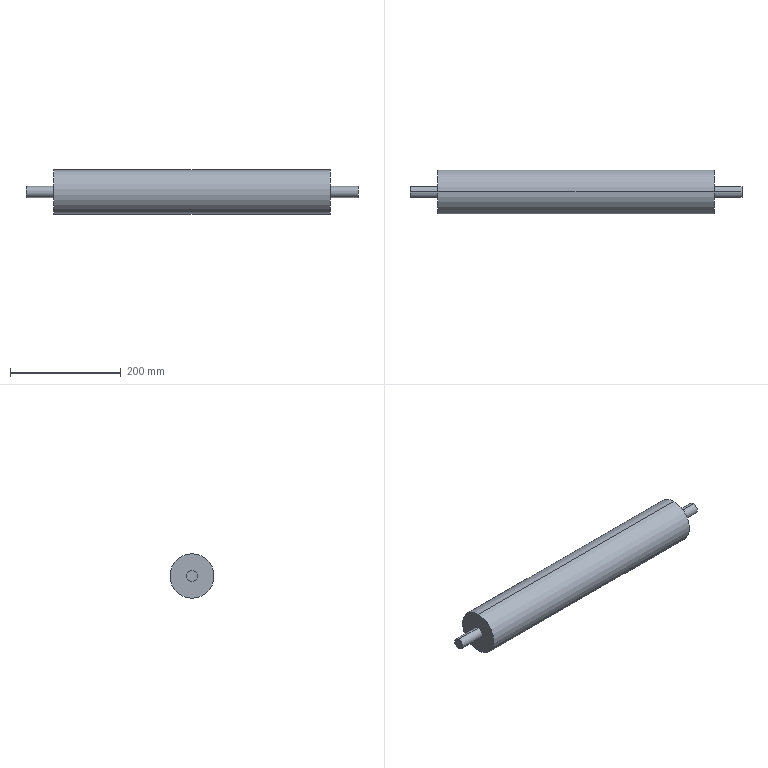Part | SolidWorks | features Revolution 1 | 1 solid | 10 faces | box 600 x 80 x 80 mm | volume 2544690 mm3 | cylinder 6 | plane 4 | commonest cylinder face diameters 20 x4 80 x2
STEP:
#1=CARTESIAN_POINT('',(-173.025,190.414,10.));
#2=VERTEX_POINT('',#1);
#3=CARTESIAN_POINT('',(-173.025,190.414,-10.));
#4=VERTEX_POINT('',#3);
#5=CARTESIAN_POINT('',(-173.025,190.414,0.));
#6=DIRECTION('',(-1.,0.,0.));
#7=DIRECTION('',(0.,0.,1.));
#8=AXIS2_PLACEMENT_3D('',#5,#6,#7);
#9=CIRCLE('',#8,10.);
#10=EDGE_CURVE('',#2,#4,#9,.T.);
#11=ORIENTED_EDGE('',*,*,#10,.T.);
#12=CARTESIAN_POINT('',(-223.025,190.414,-10.));
#13=VERTEX_POINT('',#12);
#14=CARTESIAN_POINT('',(-223.025,190.414,-10.));
#15=DIRECTION('',(-1.,0.,0.));
#16=VECTOR('',#15,1000.);
#17=LINE('',#14,#16);
#18=EDGE_CURVE('',#4,#13,#17,.T.);
#19=ORIENTED_EDGE('',*,*,#18,.T.);
#20=CARTESIAN_POINT('',(-223.025,190.414,10.));
#21=VERTEX_POINT('',#20);
#22=CARTESIAN_POINT('',(-223.025,190.414,0.));
#23=DIRECTION('',(-1.,0.,0.));
#24=DIRECTION('',(0.,0.,1.));
#25=AXIS2_PLACEMENT_3D('',#22,#23,#24);
#26=CIRCLE('',#25,10.);
#27=EDGE_CURVE('',#21,#13,#26,.T.);
#28=ORIENTED_EDGE('',*,*,#27,.F.);
#29=CARTESIAN_POINT('',(-223.025,190.414,10.));
#30=DIRECTION('',(-1.,0.,0.));
#31=VECTOR('',#30,1000.);
#32=LINE('',#29,#31);
#33=EDGE_CURVE('',#2,#21,#32,.T.);
#34=ORIENTED_EDGE('',*,*,#33,.F.);
#35=EDGE_LOOP('',(#11,#19,#28,#34));
#36=FACE_OUTER_BOUND('',#35,.T.);
#37=CARTESIAN_POINT('',(-223.025,190.414,0.));
#38=DIRECTION('',(-1.,0.,0.));
#39=DIRECTION('',(0.,0.,1.));
#40=AXIS2_PLACEMENT_3D('',#37,#38,#39);
#41=CYLINDRICAL_SURFACE('',#40,10.);
#42=ADVANCED_FACE('',(#36),#41,.T.);
#43=CARTESIAN_POINT('',(326.975,190.414,40.));
#44=VERTEX_POINT('',#43);
#45=CARTESIAN_POINT('',(326.975,190.414,-40.));
#46=VERTEX_POINT('',#45);
#47=CARTESIAN_POINT('',(326.975,190.414,0.));
#48=DIRECTION('',(-1.,0.,0.));
#49=DIRECTION('',(0.,0.,1.));
#50=AXIS2_PLACEMENT_3D('',#47,#48,#49);
#51=CIRCLE('',#50,40.);
#52=EDGE_CURVE('',#44,#46,#51,.T.);
#53=ORIENTED_EDGE('',*,*,#52,.T.);
#54=CARTESIAN_POINT('',(-173.025,190.414,-40.));
#55=VERTEX_POINT('',#54);
#56=CARTESIAN_POINT('',(-223.025,190.414,-40.));
#57=DIRECTION('',(-1.,0.,0.));
#58=VECTOR('',#57,1000.);
#59=LINE('',#56,#58);
#60=EDGE_CURVE('',#46,#55,#59,.T.);
#61=ORIENTED_EDGE('',*,*,#60,.T.);
#62=CARTESIAN_POINT('',(-173.025,190.414,40.));
#63=VERTEX_POINT('',#62);
#64=CARTESIAN_POINT('',(-173.025,190.414,0.));
#65=DIRECTION('',(-1.,0.,0.));
#66=DIRECTION('',(0.,0.,1.));
#67=AXIS2_PLACEMENT_3D('',#64,#65,#66);
#68=CIRCLE('',#67,40.);
#69=EDGE_CURVE('',#63,#55,#68,.T.);
#70=ORIENTED_EDGE('',*,*,#69,.F.);
#71=CARTESIAN_POINT('',(-223.025,190.414,40.));
#72=DIRECTION('',(-1.,0.,0.));
#73=VECTOR('',#72,1000.);
#74=LINE('',#71,#73);
#75=EDGE_CURVE('',#44,#63,#74,.T.);
#76=ORIENTED_EDGE('',*,*,#75,.F.);
#77=EDGE_LOOP('',(#53,#61,#70,#76));
#78=FACE_OUTER_BOUND('',#77,.T.);
#79=CARTESIAN_POINT('',(-223.025,190.414,0.));
#80=DIRECTION('',(-1.,0.,0.));
#81=DIRECTION('',(0.,0.,1.));
#82=AXIS2_PLACEMENT_3D('',#79,#80,#81);
#83=CYLINDRICAL_SURFACE('',#82,40.);
#84=ADVANCED_FACE('',(#78),#83,.T.);
#85=CARTESIAN_POINT('',(376.975,190.414,10.));
#86=VERTEX_POINT('',#85);
#87=CARTESIAN_POINT('',(376.975,190.414,-10.));
#88=VERTEX_POINT('',#87);
#89=CARTESIAN_POINT('',(376.975,190.414,0.));
#90=DIRECTION('',(-1.,0.,0.));
#91=DIRECTION('',(0.,0.,1.));
#92=AXIS2_PLACEMENT_3D('',#89,#90,#91);
#93=CIRCLE('',#92,10.);
#94=EDGE_CURVE('',#86,#88,#93,.T.);
#95=ORIENTED_EDGE('',*,*,#94,.T.);
#96=CARTESIAN_POINT('',(326.975,190.414,-10.));
#97=VERTEX_POINT('',#96);
#98=CARTESIAN_POINT('',(-223.025,190.414,-10.));
#99=DIRECTION('',(-1.,0.,0.));
#100=VECTOR('',#99,1000.);
#101=LINE('',#98,#100);
#102=EDGE_CURVE('',#88,#97,#101,.T.);
#103=ORIENTED_EDGE('',*,*,#102,.T.);
#104=CARTESIAN_POINT('',(326.975,190.414,10.));
#105=VERTEX_POINT('',#104);
#106=CARTESIAN_POINT('',(326.975,190.414,0.));
#107=DIRECTION('',(-1.,0.,0.));
#108=DIRECTION('',(0.,0.,1.));
#109=AXIS2_PLACEMENT_3D('',#106,#107,#108);
#110=CIRCLE('',#109,10.);
#111=EDGE_CURVE('',#105,#97,#110,.T.);
#112=ORIENTED_EDGE('',*,*,#111,.F.);
#113=CARTESIAN_POINT('',(-223.025,190.414,10.));
#114=DIRECTION('',(-1.,0.,0.));
#115=VECTOR('',#114,1000.);
#116=LINE('',#113,#115);
#117=EDGE_CURVE('',#86,#105,#116,.T.);
#118=ORIENTED_EDGE('',*,*,#117,.F.);
#119=EDGE_LOOP('',(#95,#103,#112,#118));
#120=FACE_OUTER_BOUND('',#119,.T.);
#121=CARTESIAN_POINT('',(-223.025,190.414,0.));
#122=DIRECTION('',(-1.,0.,0.));
#123=DIRECTION('',(0.,0.,1.));
#124=AXIS2_PLACEMENT_3D('',#121,#122,#123);
#125=CYLINDRICAL_SURFACE('',#124,10.);
#126=ADVANCED_FACE('',(#120),#125,.T.);
#127=ORIENTED_EDGE('',*,*,#27,.T.);
#128=CARTESIAN_POINT('',(-223.025,190.414,0.));
#129=DIRECTION('',(-1.,0.,0.));
#130=DIRECTION('',(0.,0.,1.));
#131=AXIS2_PLACEMENT_3D('',#128,#129,#130);
#132=CIRCLE('',#131,10.);
#133=EDGE_CURVE('',#13,#21,#132,.T.);
#134=ORIENTED_EDGE('',*,*,#133,.T.);
#135=EDGE_LOOP('',(#127,#134));
#136=FACE_OUTER_BOUND('',#135,.T.);
#137=CARTESIAN_POINT('',(-223.025,200.414,0.));
#138=DIRECTION('',(1.,0.,0.));
#139=DIRECTION('',(0.,0.,-1.));
#140=AXIS2_PLACEMENT_3D('',#137,#138,#139);
#141=PLANE('',#140);
#142=ADVANCED_FACE('',(#136),#141,.F.);
#143=ORIENTED_EDGE('',*,*,#94,.F.);
#144=CARTESIAN_POINT('',(376.975,190.414,0.));
#145=DIRECTION('',(-1.,0.,0.));
#146=DIRECTION('',(0.,0.,1.));
#147=AXIS2_PLACEMENT_3D('',#144,#145,#146);
#148=CIRCLE('',#147,10.);
#149=EDGE_CURVE('',#88,#86,#148,.T.);
#150=ORIENTED_EDGE('',*,*,#149,.F.);
#151=EDGE_LOOP('',(#143,#150));
#152=FACE_OUTER_BOUND('',#151,.T.);
#153=CARTESIAN_POINT('',(376.975,190.414,0.));
#154=DIRECTION('',(-1.,0.,0.));
#155=DIRECTION('',(0.,0.,1.));
#156=AXIS2_PLACEMENT_3D('',#153,#154,#155);
#157=PLANE('',#156);
#158=ADVANCED_FACE('',(#152),#157,.F.);
#159=ORIENTED_EDGE('',*,*,#102,.F.);
#160=ORIENTED_EDGE('',*,*,#149,.T.);
#161=ORIENTED_EDGE('',*,*,#117,.T.);
#162=CARTESIAN_POINT('',(326.975,190.414,0.));
#163=DIRECTION('',(-1.,0.,0.));
#164=DIRECTION('',(0.,0.,1.));
#165=AXIS2_PLACEMENT_3D('',#162,#163,#164);
#166=CIRCLE('',#165,10.);
#167=EDGE_CURVE('',#97,#105,#166,.T.);
#168=ORIENTED_EDGE('',*,*,#167,.F.);
#169=EDGE_LOOP('',(#159,#160,#161,#168));
#170=FACE_OUTER_BOUND('',#169,.T.);
#171=CARTESIAN_POINT('',(-223.025,190.414,0.));
#172=DIRECTION('',(-1.,0.,0.));
#173=DIRECTION('',(0.,0.,1.));
#174=AXIS2_PLACEMENT_3D('',#171,#172,#173);
#175=CYLINDRICAL_SURFACE('',#174,10.);
#176=ADVANCED_FACE('',(#170),#175,.T.);
#177=ORIENTED_EDGE('',*,*,#52,.F.);
#178=CARTESIAN_POINT('',(326.975,190.414,0.));
#179=DIRECTION('',(-1.,0.,0.));
#180=DIRECTION('',(0.,0.,1.));
#181=AXIS2_PLACEMENT_3D('',#178,#179,#180);
#182=CIRCLE('',#181,40.);
#183=EDGE_CURVE('',#46,#44,#182,.T.);
#184=ORIENTED_EDGE('',*,*,#183,.F.);
#185=EDGE_LOOP('',(#177,#184));
#186=FACE_OUTER_BOUND('',#185,.T.);
#187=ORIENTED_EDGE('',*,*,#111,.T.);
#188=ORIENTED_EDGE('',*,*,#167,.T.);
#189=EDGE_LOOP('',(#187,#188));
#190=FACE_BOUND('',#189,.T.);
#191=CARTESIAN_POINT('',(326.975,200.414,0.));
#192=DIRECTION('',(-1.,0.,0.));
#193=DIRECTION('',(0.,0.,1.));
#194=AXIS2_PLACEMENT_3D('',#191,#192,#193);
#195=PLANE('',#194);
#196=ADVANCED_FACE('',(#186,#190),#195,.F.);
#197=ORIENTED_EDGE('',*,*,#60,.F.);
#198=ORIENTED_EDGE('',*,*,#183,.T.);
#199=ORIENTED_EDGE('',*,*,#75,.T.);
#200=CARTESIAN_POINT('',(-173.025,190.414,0.));
#201=DIRECTION('',(-1.,0.,0.));
#202=DIRECTION('',(0.,0.,1.));
#203=AXIS2_PLACEMENT_3D('',#200,#201,#202);
#204=CIRCLE('',#203,40.);
#205=EDGE_CURVE('',#55,#63,#204,.T.);
#206=ORIENTED_EDGE('',*,*,#205,.F.);
#207=EDGE_LOOP('',(#197,#198,#199,#206));
#208=FACE_OUTER_BOUND('',#207,.T.);
#209=CARTESIAN_POINT('',(-223.025,190.414,0.));
#210=DIRECTION('',(-1.,0.,0.));
#211=DIRECTION('',(0.,0.,1.));
#212=AXIS2_PLACEMENT_3D('',#209,#210,#211);
#213=CYLINDRICAL_SURFACE('',#212,40.);
#214=ADVANCED_FACE('',(#208),#213,.T.);
#215=ORIENTED_EDGE('',*,*,#10,.F.);
#216=CARTESIAN_POINT('',(-173.025,190.414,0.));
#217=DIRECTION('',(-1.,0.,0.));
#218=DIRECTION('',(0.,0.,1.));
#219=AXIS2_PLACEMENT_3D('',#216,#217,#218);
#220=CIRCLE('',#219,10.);
#221=EDGE_CURVE('',#4,#2,#220,.T.);
#222=ORIENTED_EDGE('',*,*,#221,.F.);
#223=EDGE_LOOP('',(#215,#222));
#224=FACE_BOUND('',#223,.T.);
#225=ORIENTED_EDGE('',*,*,#69,.T.);
#226=ORIENTED_EDGE('',*,*,#205,.T.);
#227=EDGE_LOOP('',(#225,#226));
#228=FACE_OUTER_BOUND('',#227,.T.);
#229=CARTESIAN_POINT('',(-173.025,230.414,0.));
#230=DIRECTION('',(1.,0.,0.));
#231=DIRECTION('',(0.,0.,-1.));
#232=AXIS2_PLACEMENT_3D('',#229,#230,#231);
#233=PLANE('',#232);
#234=ADVANCED_FACE('',(#224,#228),#233,.F.);
#235=ORIENTED_EDGE('',*,*,#18,.F.);
#236=ORIENTED_EDGE('',*,*,#221,.T.);
#237=ORIENTED_EDGE('',*,*,#33,.T.);
#238=ORIENTED_EDGE('',*,*,#133,.F.);
#239=EDGE_LOOP('',(#235,#236,#237,#238));
#240=FACE_OUTER_BOUND('',#239,.T.);
#241=CARTESIAN_POINT('',(-223.025,190.414,0.));
#242=DIRECTION('',(-1.,0.,0.));
#243=DIRECTION('',(0.,0.,1.));
#244=AXIS2_PLACEMENT_3D('',#241,#242,#243);
#245=CYLINDRICAL_SURFACE('',#244,10.);
#246=ADVANCED_FACE('',(#240),#245,.T.);
#247=CLOSED_SHELL('',(#42,#84,#126,#142,#158,#176,#196,#214,#234,#246));
#248=MANIFOLD_SOLID_BREP('',#247);
#249=CARTESIAN_POINT('',(0.,0.,0.));
#250=DIRECTION('',(0.,0.,1.));
#251=DIRECTION('',(1.,0.,0.));
#252=AXIS2_PLACEMENT_3D('',#249,#250,#251);
#253=(LENGTH_UNIT()NAMED_UNIT(*)SI_UNIT(.MILLI.,.METRE.));
#254=UNCERTAINTY_MEASURE_WITH_UNIT(LENGTH_MEASURE(0.00001),#253,'','');
#255=(NAMED_UNIT(*)PLANE_ANGLE_UNIT()SI_UNIT($,.RADIAN.));
#256=(NAMED_UNIT(*)SI_UNIT($,.STERADIAN.)SOLID_ANGLE_UNIT());
#257=(GEOMETRIC_REPRESENTATION_CONTEXT(3)GLOBAL_UNCERTAINTY_ASSIGNED_CONTEXT((#254))GLOBAL_UNIT_ASSIGNED_CONTEXT((#253,#255,#256))REPRESENTATION_CONTEXT('',''));
#258=ADVANCED_BREP_SHAPE_REPRESENTATION('',(#248,#252),#257);